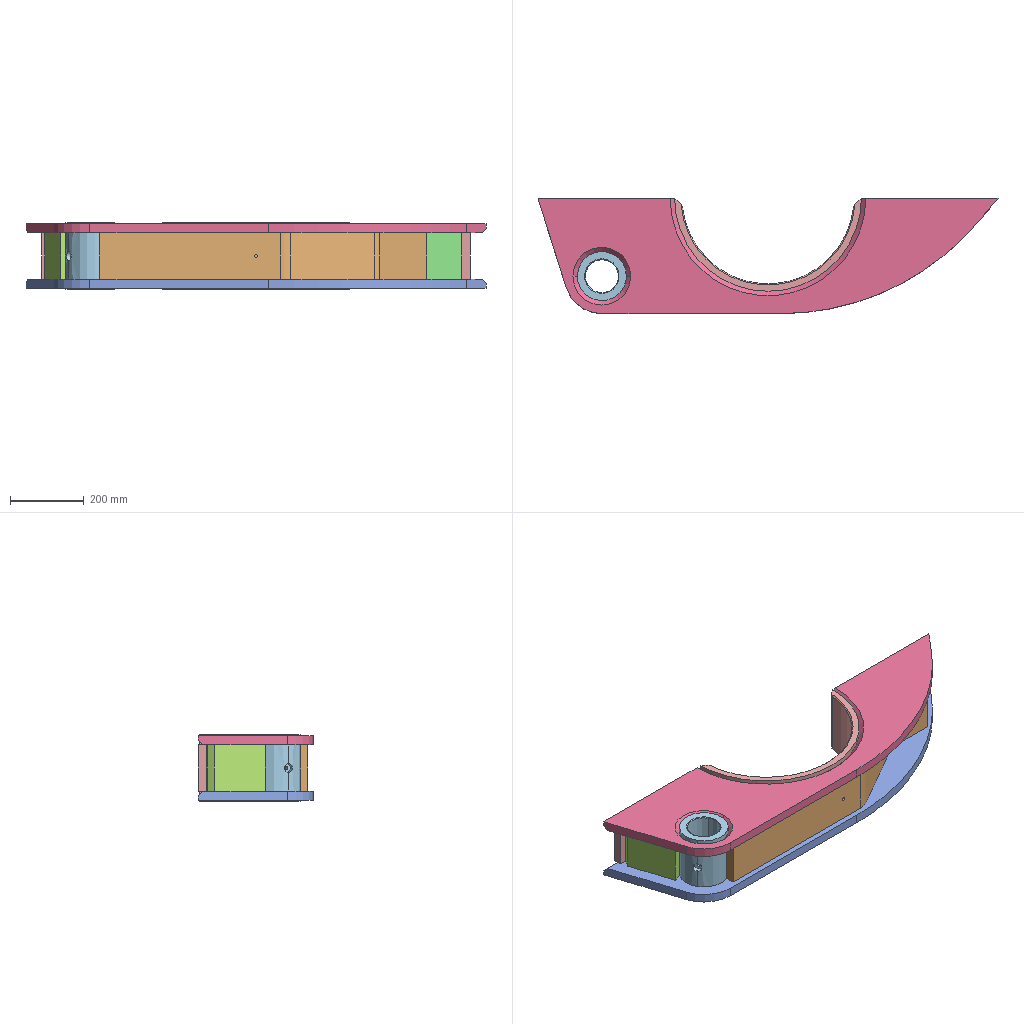Assembly | SolidWorks | 10 different items | 10 placed | box 1246 x 312 x 180 mm
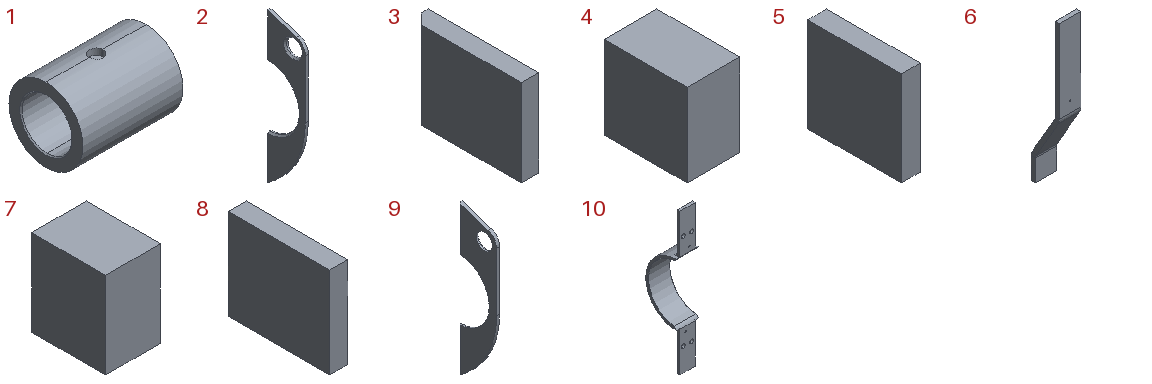Parts list (item | quantity | size | volume | features):
1 | x1 | 180 x 133 x 133 mm | 1348176 mm3 | features Chamfer 1, Extrusion 1, HoleWzd 1, ICE 1
2 | x1 | 25 x 312.3 x 1246 mm | 4938572 mm3 | features Chamfer 2, Extrusion 1, Fillet 1, ICE 1
3 | x1 | 25 x 160 x 126 mm | 489825 mm3 | features Chamfer 1, Extrusion 1
4 | x1 | 80 x 126 x 126 mm | 1136246 mm3 | features Extrusion 1, HoleWzd 1
5 | x1 | 25 x 125 x 126 mm | 393750 mm3 | features Extrusion 1
6 | x1 | 126 x 168 x 887 mm | 2910198 mm3 | features FlatPattern 1, ICE 1, SMBaseFlange 1, SheetMetal 1
7 | x1 | 80 x 108 x 126 mm | 954806 mm3 | features Extrusion 1, HoleWzd 1
8 | x1 | 25 x 141 x 126 mm | 444150 mm3 | features Extrusion 1
9 | x1 | 25 x 312.3 x 1246 mm | 4938572 mm3 | features Chamfer 2, Extrusion 1, Fillet 1, ICE 1
10 | x1 | 180 x 251.8 x 1160 mm | 4341383 mm3 | features ICE 4, Fillet 2, MirrorPattern 2, Chamfer 1, Extrusion 1, HoleWzd 1
Mates (type | each side: item.copy, entity, surface, feature):
Coincident | 10.1 plane | assembly plane | 3 times
Coincident | 10.1 face plane Boss-Extrude1 | 3.1 edge
Coincident | 3.1 plane | assembly plane
DistanceDim | 4.1 plane | assembly plane
Coincident | 10.1 face plane Boss-Extrude1 | 4.1 face plane Boss-Extrude1
DistanceDim | 5.1 face plane Boss-Extrude1 | assembly plane
Coincident | 6.1 plane | assembly plane | 2 times
DistanceDim | 7.1 plane | assembly plane
Coincident | 10.1 face plane Boss-Extrude1 | 7.1 face plane Boss-Extrude1
Coincident | 10.1 face plane Boss-Extrude1 | 8.1 edge
Coincident | 8.1 plane | assembly plane
DistanceDim | assembly plane | 9.1 face plane Boss-Extrude1
Coincident | 9.1 plane | assembly plane | 2 times
PlanarAngleDim | 1.1 plane | assembly plane
DistanceDim | 2.1 face plane Boss-Extrude1 | assembly plane
Coincident | 2.1 plane | assembly plane | 2 times
DistanceDim | 3.1 face plane Boss-Extrude1 | 2.1 face plane Boss-Extrude1
Coincident | 4.1 plane | assembly plane
Coincident | 5.1 plane | assembly plane
Coincident | 4.1 face plane Boss-Extrude1 | 5.1 face plane Boss-Extrude1
Coincident | 5.1 face plane Boss-Extrude1 | 6.1 face plane Base-Flange1
Coincident | 7.1 plane | assembly plane
Coincident | 7.1 face plane Boss-Extrude1 | 8.1 edge
Coincident | 6.1 face plane Base-Flange1 | 8.1 edge
Coincident | 1.1 plane | assembly plane
Concentric | 2.1 face cylinder Cut-Extrude1 | 1.1 face cylinder Boss-Extrude1